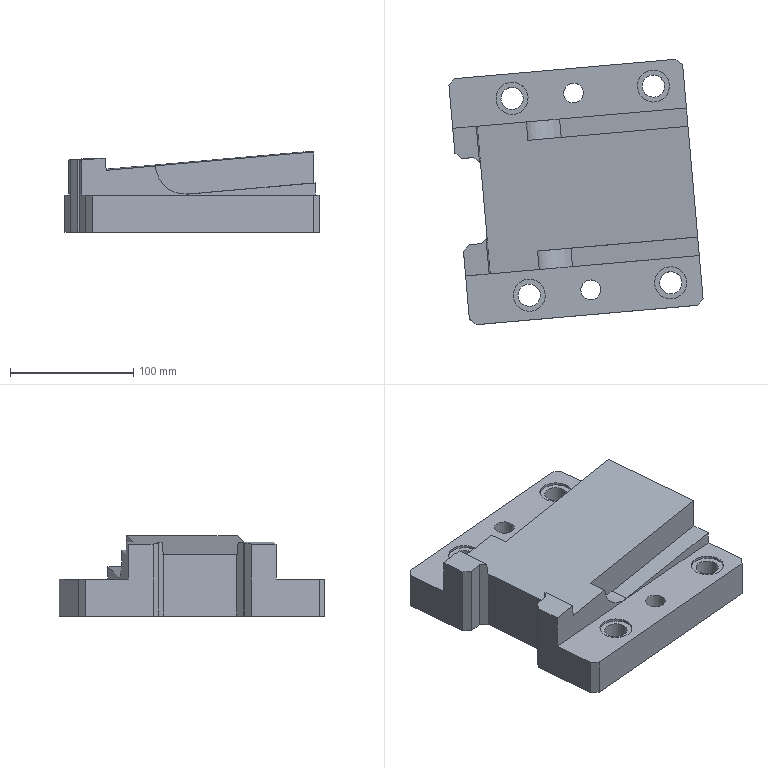Part | NX | features solid 2 | 1 solid | 67 faces | box 205.837 x 214.927 x 64.873 mm | volume 1492190 mm3 | plane 55 | cylinder 12 | commonest cylinder face diameters 18 x4 26 x4 16 x2 50 x2